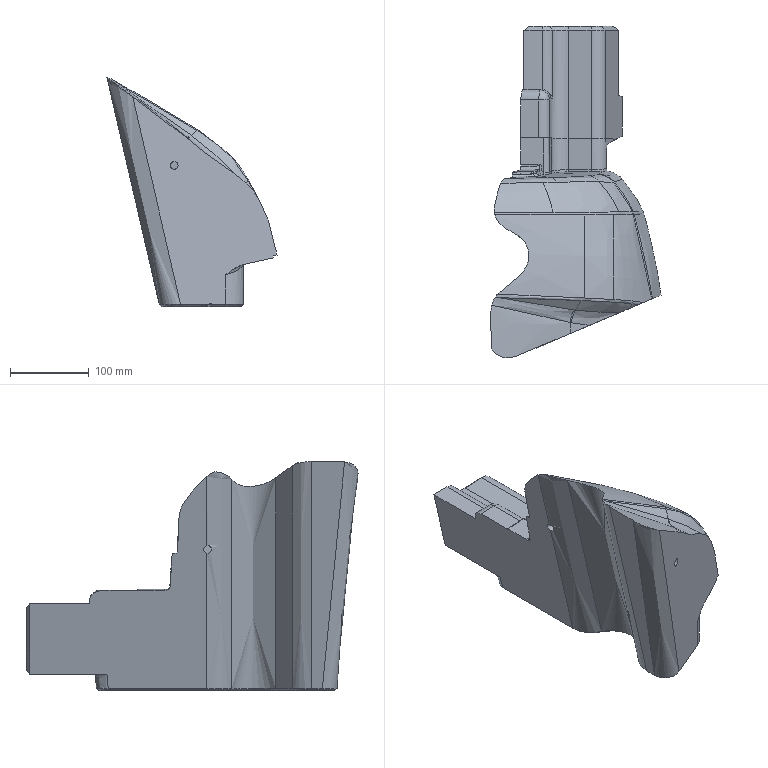Part | STEP file | solid 61 | 1 solid | 191 faces | box 215.526 x 420.609 x 290.404 mm | volume 6488252 mm3 | spline 114 | plane 34 | cylinder 34 | cone 7 | other 1 | sphere 1 | commonest cylinder face diameters 10 x15 30 x6 26 x3 14 x2 36.468 x2 40.52 x2